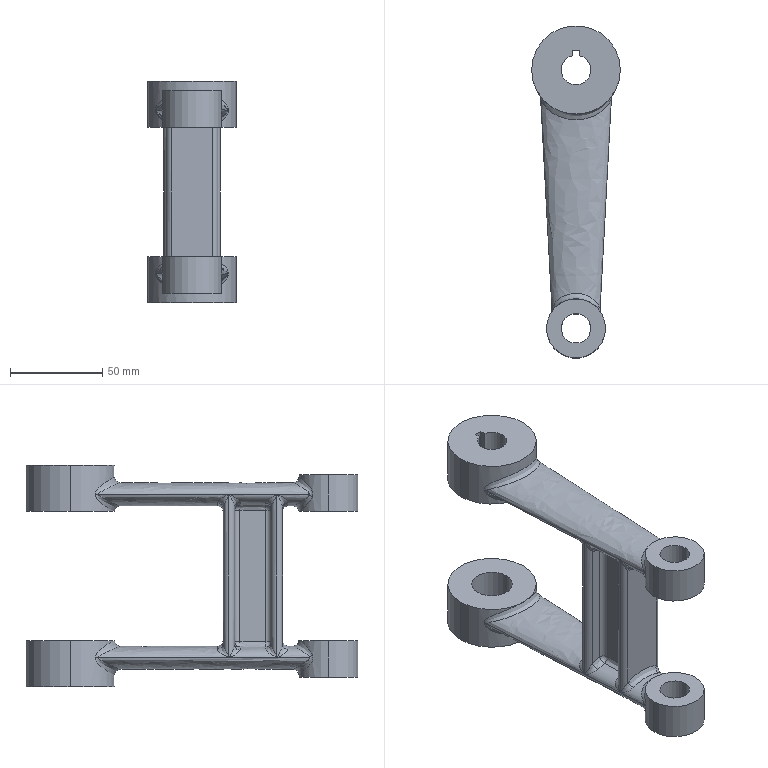Part | SolidWorks | features ICE 3, Blend 1, Extrusion 1, Fillet 1, MirrorSolid 1, Sculpt 1 | 1 solid | 93 faces | box 48 x 180 x 120 mm | volume 202077 mm3 | spline 36 | cylinder 28 | plane 19 | sphere 10 | commonest cylinder face diameters 16 x7 6 x6 32 x4 48 x4 6.087 x2 6.097 x2